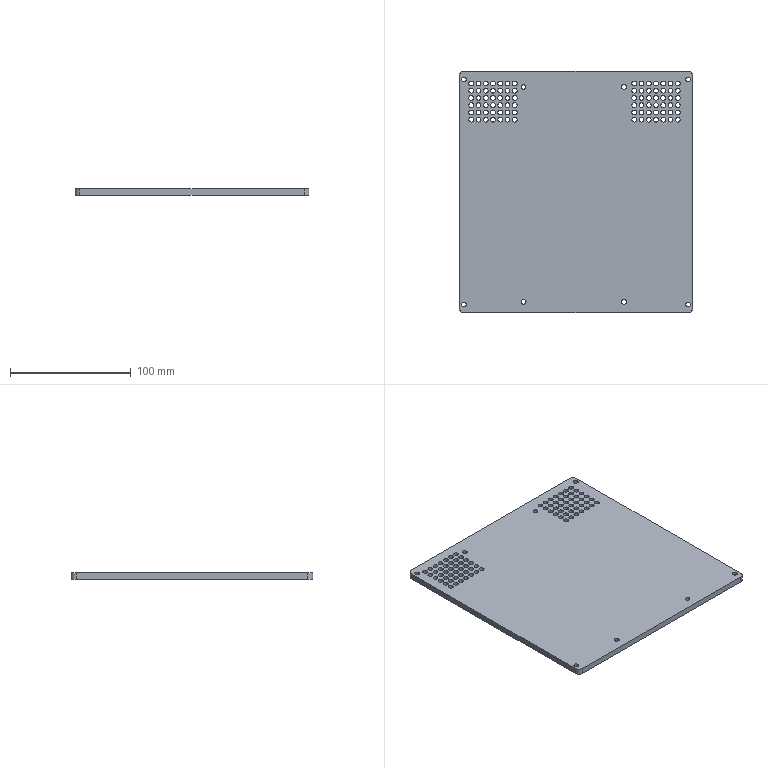Part | SolidWorks | features ICE 3, Extrusion 1, Fillet 1, LPattern 1 | 1 solid | 194 faces | box 193.6 x 200 x 5 mm | volume 187754 mm3 | cylinder 188 | plane 6 | commonest cylinder face diameters 4 x182 8 x4 3.905 x2